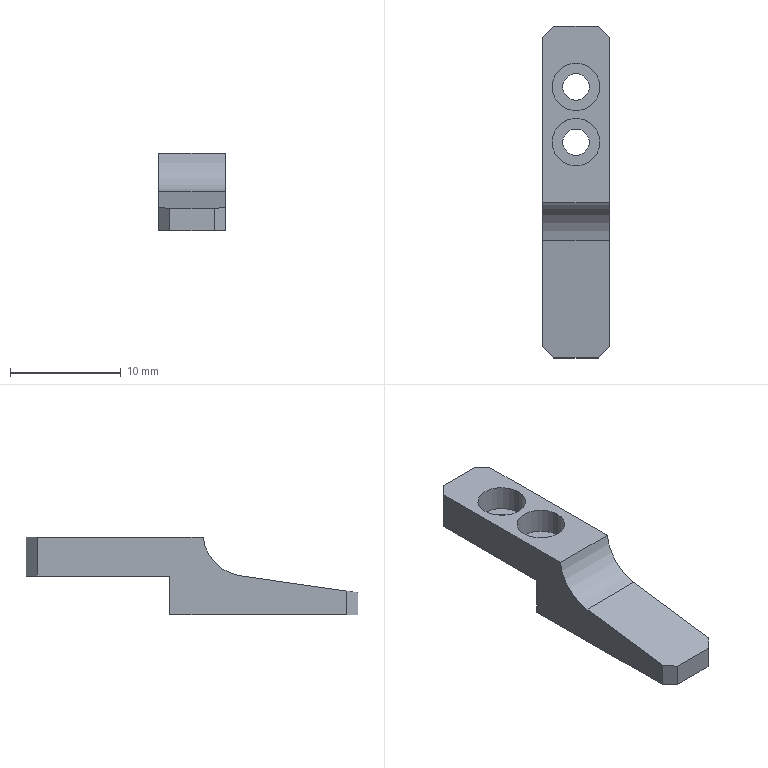Part | STEP file | 0-19-07 Finger 2 | 1 solid | 24 faces | box 6 x 30 x 7 mm | volume 581.935 mm3 | plane 15 | cylinder 9 | commonest cylinder face diameters 2.4 x4 4.3 x4 8 x1